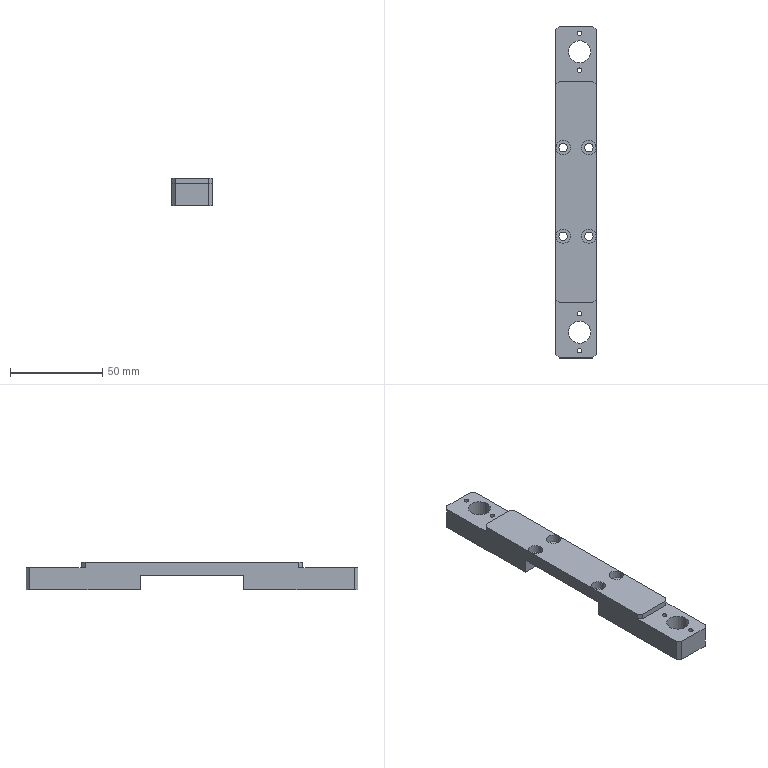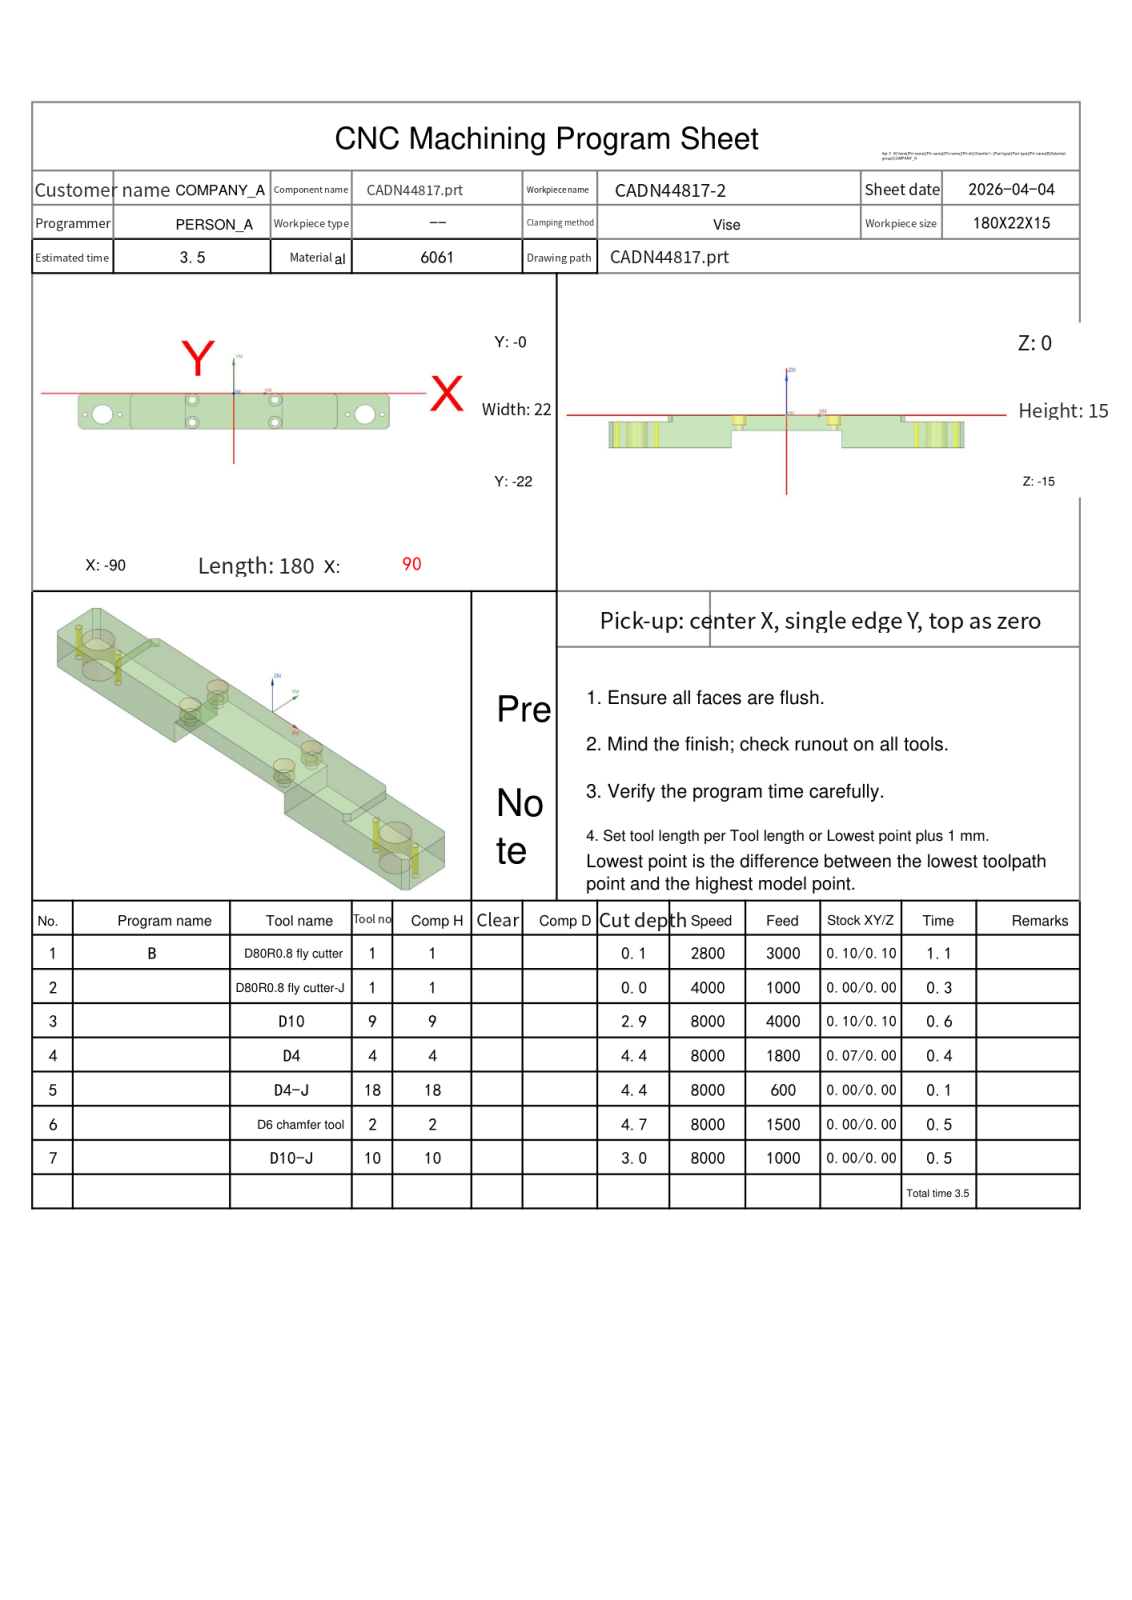NC program | NX | posted by the shop | part box 22 x 180 x 15 mm
Whole program:
%
O0001
(Machine time: 4.85 MIN)
(===Total Tool:6===)
(T1=D80R0.8 fly cutter D=80. R=0.8 D- H01 Z=-0.   )
(T9=D10     D=10.  R=0.   D-  H09 Z=-2.9  )
(T4=D4      D=4.   R=0.   D-  H04 Z=-4.4  )
(T18=D4-J   D=4.   R=0.   D-  H18 Z=-4.4  )
(T2=D6 chamfer tool D=6. R=0. D- H02 Z=-4.75 )
(T10=D10-J  D=10.  R=0.   D10 H10 Z=-3.   )
G80 G90 G17 G49 G40
G91 G28 Z0
M01
N1 T01 M06
(D80R0.8 fly cutter D=80. R=0.8 H=01 ce=0.10 di=0.10)
G00 G90 G54 X-142.097 Y-11. M03 S2800
G43 H01 Z20.
M08
Z6.011
G01 Z4.011 F3000.
X-130.097
X130.097
X142.097
Z6.011
G00 X-142.097
Z5.522
G01 Z3.522
X-130.097
X130.097
X142.097
Z5.522
G00 X-142.097
Z5.033
G01 Z3.033
X-130.097
X130.097
X142.097
Z5.033
G00 X-142.097
Z4.544
G01 Z2.544
X-130.097
X130.097
X142.097
Z4.544
G00 Z20.
X-142.097
Z4.056
G01 Z2.056
X-130.097
X130.097
X142.097
Z4.056
G00 Z20.
X-142.097
Z3.567
G01 Z1.567
X-130.097
X130.097
X142.097
Z3.567
G00 Z20.
X-142.097
Z3.078
G01 Z1.078
X-130.097
X130.097
X142.097
Z3.078
G00 Z20.
X-142.097
Z2.589
G01 Z.589
X-130.097
X130.097
X142.097
Z2.589
G00 Z20.
X-142.097
Z2.1
G01 Z.1
X-130.097
X130.097
X142.097
Z2.1
G00 Z20.
G91 G28 Z0.0
M05
M09
G91 G28 Z0.0
M01
N2 T01 M06
(D80R0.8 fly cutter-J D=80. R=0.8 H=01 ce=0.00 di=0.00)
G00 G90 G54 X-141.999 Y-11. M03 S4000
G43 H01 Z20.
M08
Z2.
G01 Z0.0 F1000.
X-129.999
X129.999
X141.999
Z2.
G00 Z20.
G91 G28 Z0.0
M05
M09
G91 G28 Z0.0
M01
N3 T09 M06
(D10  D=10. R=0. H=09 ce=0.10 di=0.10)
G00 G90 G54 X-92.099 Y-29.209 M03 S8000
G43 H09 Z14.5
M08
Z.92
G01 Z-.58 F4000.
X-92.502 Y-24.427
G02 X-92.6 Y-22.114 I27.402 J2.315
G01 Y.112
G02 X-92.531 Y2.052 I27.5 J0.0
X-92.241 Y2.688 I.997 J-.071
G01 X-90.322 Y4.607
G02 X-89.616 Y4.9 I.707 J-.707
G01 X-88.056
G02 X-87.256 Y4.1 I0.0 J-.8
G01 X-87.268 Y3.963
G03 X-87.6 Y.112 I22.168 J-3.851
G01 Y-22.114
G03 X-87.248 Y-26.076 I22.5 J.002
X-86.264 Y-26.9 I.984 J.176
G01 X-80.258
G03 X-79.559 Y-26.2 I0.0 J.7
G01 X-79.583 Y-26.018
G02 X-80.1 Y-22.114 I14.483 J3.906
G01 Y.112
G02 X-79.541 Y4.171 I15. J0.0
X-78.578 Y4.9 I.963 J-.271
G01 X-71.854
G02 X-71.354 Y4.4 I0.0 J-.5
X-71.432 Y4.132 I-.5 J0.0
G03 X-72.6 Y.112 I6.332 J-4.02
G01 Y-22.112
G03 X-71.127 Y-26.576 I7.5 J0.0
X-70.496 Y-26.966 I.803 J.595
G01 X-61.192 Y-28.592
X-61.02 Y-28.607
G03 X-60.02 Y-27.607 I0.0 J1.
X-60.312 Y-26.9 I-1. J0.0
G01 X-65.1 Y-22.112
Y.112
X-60.312 Y4.9
X-57.112 Y8.1
Z.92
G00 Z14.5
X-92.099 Y-29.209
Z.34
G01 Z-1.16
X-92.502 Y-24.427
G02 X-92.6 Y-22.114 I27.402 J2.315
G01 Y.112
G02 X-92.531 Y2.052 I27.5 J0.0
X-92.241 Y2.688 I.997 J-.071
G01 X-90.322 Y4.607
G02 X-89.616 Y4.9 I.707 J-.707
G01 X-88.056
G02 X-87.256 Y4.1 I0.0 J-.8
G01 X-87.268 Y3.963
G03 X-87.6 Y.112 I22.168 J-3.851
G01 Y-22.114
G03 X-87.248 Y-26.076 I22.5 J.002
X-86.264 Y-26.9 I.984 J.176
G01 X-80.258
G03 X-79.559 Y-26.2 I0.0 J.7
G01 X-79.583 Y-26.018
G02 X-80.1 Y-22.114 I14.483 J3.906
G01 Y.112
G02 X-79.541 Y4.171 I15. J0.0
X-78.578 Y4.9 I.963 J-.271
G01 X-71.854
G02 X-71.354 Y4.4 I0.0 J-.5
X-71.432 Y4.132 I-.5 J0.0
G03 X-72.6 Y.112 I6.332 J-4.02
G01 Y-22.112
G03 X-71.127 Y-26.576 I7.5 J0.0
X-70.496 Y-26.966 I.803 J.595
G01 X-61.192 Y-28.592
X-61.02 Y-28.607
G03 X-60.02 Y-27.607 I0.0 J1.
X-60.312 Y-26.9 I-1. J0.0
G01 X-65.1 Y-22.112
Y.112
X-60.312 Y4.9
X-57.112 Y8.1
Z.34
G00 Z14.5
X-92.099 Y-29.209
Z-.24
G01 Z-1.74
X-92.502 Y-24.427
G02 X-92.6 Y-22.114 I27.402 J2.315
G01 Y.112
G02 X-92.531 Y2.052 I27.5 J0.0
X-92.241 Y2.688 I.997 J-.071
G01 X-90.322 Y4.607
G02 X-89.616 Y4.9 I.707 J-.707
G01 X-88.056
G02 X-87.256 Y4.1 I0.0 J-.8
G01 X-87.268 Y3.963
G03 X-87.6 Y.112 I22.168 J-3.851
G01 Y-22.114
G03 X-87.248 Y-26.076 I22.5 J.002
X-86.264 Y-26.9 I.984 J.176
G01 X-80.258
G03 X-79.559 Y-26.2 I0.0 J.7
G01 X-79.583 Y-26.018
G02 X-80.1 Y-22.114 I14.483 J3.906
G01 Y.112
G02 X-79.541 Y4.171 I15. J0.0
X-78.578 Y4.9 I.963 J-.271
G01 X-71.854
G02 X-71.354 Y4.4 I0.0 J-.5
X-71.432 Y4.132 I-.5 J0.0
G03 X-72.6 Y.112 I6.332 J-4.02
G01 Y-22.112
G03 X-71.127 Y-26.576 I7.5 J0.0
X-70.496 Y-26.966 I.803 J.595
G01 X-61.192 Y-28.592
X-61.02 Y-28.607
G03 X-60.02 Y-27.607 I0.0 J1.
X-60.312 Y-26.9 I-1. J0.0
G01 X-65.1 Y-22.112
Y.112
X-60.312 Y4.9
X-57.112 Y8.1
Z-.24
G00 Z14.5
X-92.099 Y-29.209
Z-.82
G01 Z-2.32
X-92.502 Y-24.427
G02 X-92.6 Y-22.114 I27.402 J2.315
G01 Y.112
G02 X-92.531 Y2.052 I27.5 J0.0
X-92.241 Y2.688 I.997 J-.071
G01 X-90.322 Y4.607
G02 X-89.616 Y4.9 I.707 J-.707
G01 X-88.056
G02 X-87.256 Y4.1 I0.0 J-.8
G01 X-87.268 Y3.963
G03 X-87.6 Y.112 I22.168 J-3.851
G01 Y-22.114
G03 X-87.248 Y-26.076 I22.5 J.002
X-86.264 Y-26.9 I.984 J.176
G01 X-80.258
G03 X-79.559 Y-26.2 I0.0 J.7
G01 X-79.583 Y-26.018
G02 X-80.1 Y-22.114 I14.483 J3.906
G01 Y.112
G02 X-79.541 Y4.171 I15. J0.0
X-78.578 Y4.9 I.963 J-.271
G01 X-71.854
G02 X-71.354 Y4.4 I0.0 J-.5
X-71.432 Y4.132 I-.5 J0.0
G03 X-72.6 Y.112 I6.332 J-4.02
G01 Y-22.112
G03 X-71.127 Y-26.576 I7.5 J0.0
X-70.496 Y-26.966 I.803 J.595
G01 X-61.192 Y-28.592
X-61.02 Y-28.607
G03 X-60.02 Y-27.607 I0.0 J1.
X-60.312 Y-26.9 I-1. J0.0
G01 X-65.1 Y-22.112
Y.112
X-60.312 Y4.9
X-57.112 Y8.1
Z-.82
G00 Z14.5
X-92.099 Y-29.209
Z-1.4
G01 Z-2.9
X-92.502 Y-24.427
G02 X-92.6 Y-22.114 I27.402 J2.315
G01 Y.112
G02 X-92.531 Y2.052 I27.5 J0.0
X-92.241 Y2.688 I.997 J-.071
G01 X-90.322 Y4.607
G02 X-89.616 Y4.9 I.707 J-.707
G01 X-88.056
G02 X-87.256 Y4.1 I0.0 J-.8
G01 X-87.268 Y3.963
G03 X-87.6 Y.112 I22.168 J-3.851
G01 Y-22.114
G03 X-87.248 Y-26.076 I22.5 J.002
X-86.264 Y-26.9 I.984 J.176
G01 X-80.258
G03 X-79.559 Y-26.2 I0.0 J.7
G01 X-79.583 Y-26.018
G02 X-80.1 Y-22.114 I14.483 J3.906
G01 Y.112
G02 X-79.541 Y4.171 I15. J0.0
X-78.578 Y4.9 I.963 J-.271
G01 X-71.854
G02 X-71.354 Y4.4 I0.0 J-.5
X-71.432 Y4.132 I-.5 J0.0
G03 X-72.6 Y.112 I6.332 J-4.02
G01 Y-22.112
G03 X-71.127 Y-26.576 I7.5 J0.0
X-70.496 Y-26.966 I.803 J.595
G01 X-61.192 Y-28.592
X-61.02 Y-28.607
G03 X-60.02 Y-27.607 I0.0 J1.
X-60.312 Y-26.9 I-1. J0.0
G01 X-65.1 Y-22.112
Y.112
X-60.312 Y4.9
X-57.112 Y8.1
Z-1.4
G00 Z3.
X92.099 Y7.209
Z.92
G01 Z-.58
X92.502 Y2.427
G02 X92.6 Y.114 I-27.402 J-2.315
G01 Y-22.112
G02 X92.531 Y-24.052 I-27.5 J0.0
X92.241 Y-24.688 I-.997 J.071
G01 X90.322 Y-26.607
G02 X89.616 Y-26.9 I-.707 J.707
G01 X88.056
G02 X87.256 Y-26.1 I0.0 J.8
G01 X87.268 Y-25.963
G03 X87.6 Y-22.112 I-22.168 J3.851
G01 Y.114
G03 X87.248 Y4.076 I-22.5 J-.002
X86.264 Y4.9 I-.984 J-.176
G01 X80.258
G03 X79.559 Y4.2 I0.0 J-.7
G01 X79.583 Y4.018
G02 X80.1 Y.114 I-14.483 J-3.906
G01 Y-22.112
G02 X79.541 Y-26.171 I-15. J0.0
X78.578 Y-26.9 I-.963 J.271
G01 X71.854
G02 X71.354 Y-26.4 I0.0 J.5
X71.432 Y-26.132 I.5 J0.0
G03 X72.6 Y-22.112 I-6.332 J4.02
G01 Y.112
G03 X71.127 Y4.576 I-7.5 J0.0
X70.496 Y4.966 I-.803 J-.595
G01 X61.192 Y6.592
X61.02 Y6.607
G03 X60.02 Y5.607 I0.0 J-1.
X60.312 Y4.9 I1. J0.0
G01 X65.1 Y.112
Y-22.112
X60.312 Y-26.9
X57.112 Y-30.1
Z.92
G00 Z14.5
X92.099 Y7.209
Z.34
G01 Z-1.16
X92.502 Y2.427
G02 X92.6 Y.114 I-27.402 J-2.315
G01 Y-22.112
G02 X92.531 Y-24.052 I-27.5 J0.0
X92.241 Y-24.688 I-.997 J.071
G01 X90.322 Y-26.607
G02 X89.616 Y-26.9 I-.707 J.707
G01 X88.056
G02 X87.256 Y-26.1 I0.0 J.8
G01 X87.268 Y-25.963
G03 X87.6 Y-22.112 I-22.168 J3.851
G01 Y.114
G03 X87.248 Y4.076 I-22.5 J-.002
X86.264 Y4.9 I-.984 J-.176
G01 X80.258
G03 X79.559 Y4.2 I0.0 J-.7
G01 X79.583 Y4.018
G02 X80.1 Y.114 I-14.483 J-3.906
G01 Y-22.112
G02 X79.541 Y-26.171 I-15. J0.0
X78.578 Y-26.9 I-.963 J.271
G01 X71.854
G02 X71.354 Y-26.4 I0.0 J.5
X71.432 Y-26.132 I.5 J0.0
G03 X72.6 Y-22.112 I-6.332 J4.02
G01 Y.112
G03 X71.127 Y4.576 I-7.5 J0.0
X70.496 Y4.966 I-.803 J-.595
G01 X61.192 Y6.592
X61.02 Y6.607
G03 X60.02 Y5.607 I0.0 J-1.
X60.312 Y4.9 I1. J0.0
G01 X65.1 Y.112
Y-22.112
X60.312 Y-26.9
X57.112 Y-30.1
Z.34
G00 Z14.5
X92.099 Y7.209
Z-.24
G01 Z-1.74
X92.502 Y2.427
G02 X92.6 Y.114 I-27.402 J-2.315
G01 Y-22.112
G02 X92.531 Y-24.052 I-27.5 J0.0
X92.241 Y-24.688 I-.997 J.071
G01 X90.322 Y-26.607
G02 X89.616 Y-26.9 I-.707 J.707
G01 X88.056
G02 X87.256 Y-26.1 I0.0 J.8
G01 X87.268 Y-25.963
G03 X87.6 Y-22.112 I-22.168 J3.851
G01 Y.114
G03 X87.248 Y4.076 I-22.5 J-.002
X86.264 Y4.9 I-.984 J-.176
G01 X80.258
G03 X79.559 Y4.2 I0.0 J-.7
G01 X79.583 Y4.018
G02 X80.1 Y.114 I-14.483 J-3.906
G01 Y-22.112
G02 X79.541 Y-26.171 I-15. J0.0
X78.578 Y-26.9 I-.963 J.271
G01 X71.854
G02 X71.354 Y-26.4 I0.0 J.5
X71.432 Y-26.132 I.5 J0.0
G03 X72.6 Y-22.112 I-6.332 J4.02
G01 Y.112
G03 X71.127 Y4.576 I-7.5 J0.0
X70.496 Y4.966 I-.803 J-.595
G01 X61.192 Y6.592
X61.02 Y6.607
G03 X60.02 Y5.607 I0.0 J-1.
X60.312 Y4.9 I1. J0.0
G01 X65.1 Y.112
Y-22.112
X60.312 Y-26.9
X57.112 Y-30.1
Z-.24
G00 Z14.5
X92.099 Y7.209
Z-.82
G01 Z-2.32
X92.502 Y2.427
G02 X92.6 Y.114 I-27.402 J-2.315
G01 Y-22.112
G02 X92.531 Y-24.052 I-27.5 J0.0
X92.241 Y-24.688 I-.997 J.071
G01 X90.322 Y-26.607
G02 X89.616 Y-26.9 I-.707 J.707
G01 X88.056
G02 X87.256 Y-26.1 I0.0 J.8
G01 X87.268 Y-25.963
G03 X87.6 Y-22.112 I-22.168 J3.851
G01 Y.114
G03 X87.248 Y4.076 I-22.5 J-.002
X86.264 Y4.9 I-.984 J-.176
G01 X80.258
G03 X79.559 Y4.2 I0.0 J-.7
G01 X79.583 Y4.018
G02 X80.1 Y.114 I-14.483 J-3.906
G01 Y-22.112
G02 X79.541 Y-26.171 I-15. J0.0
X78.578 Y-26.9 I-.963 J.271
G01 X71.854
G02 X71.354 Y-26.4 I0.0 J.5
X71.432 Y-26.132 I.5 J0.0
G03 X72.6 Y-22.112 I-6.332 J4.02
G01 Y.112
G03 X71.127 Y4.576 I-7.5 J0.0
X70.496 Y4.966 I-.803 J-.595
G01 X61.192 Y6.592
X61.02 Y6.607
G03 X60.02 Y5.607 I0.0 J-1.
X60.312 Y4.9 I1. J0.0
G01 X65.1 Y.112
Y-22.112
X60.312 Y-26.9
X57.112 Y-30.1
Z-.82
G00 Z14.5
X92.099 Y7.209
Z-1.4
G01 Z-2.9
X92.502 Y2.427
G02 X92.6 Y.114 I-27.402 J-2.315
G01 Y-22.112
G02 X92.531 Y-24.052 I-27.5 J0.0
X92.241 Y-24.688 I-.997 J.071
G01 X90.322 Y-26.607
G02 X89.616 Y-26.9 I-.707 J.707
G01 X88.056
G02 X87.256 Y-26.1 I0.0 J.8
G01 X87.268 Y-25.963
G03 X87.6 Y-22.112 I-22.168 J3.851
G01 Y.114
G03 X87.248 Y4.076 I-22.5 J-.002
X86.264 Y4.9 I-.984 J-.176
G01 X80.258
G03 X79.559 Y4.2 I0.0 J-.7
G01 X79.583 Y4.018
G02 X80.1 Y.114 I-14.483 J-3.906
G01 Y-22.112
G02 X79.541 Y-26.171 I-15. J0.0
X78.578 Y-26.9 I-.963 J.271
G01 X71.854
G02 X71.354 Y-26.4 I0.0 J.5
X71.432 Y-26.132 I.5 J0.0
G03 X72.6 Y-22.112 I-6.332 J4.02
G01 Y.112
G03 X71.127 Y4.576 I-7.5 J0.0
X70.496 Y4.966 I-.803 J-.595
G01 X61.192 Y6.592
X61.02 Y6.607
G03 X60.02 Y5.607 I0.0 J-1.
X60.312 Y4.9 I1. J0.0
G01 X65.1 Y.112
Y-22.112
X60.312 Y-26.9
X57.112 Y-30.1
Z-1.4
G00 Z14.5
G91 G28 Z0.0
M05
M09
G91 G28 Z0.0
M01
N4 T04 M06
(D4  D=4. R=0. H=04 ce=0.07 di=0.00)
G00 G90 G54 X-24. Y-4. M03 S8000
G43 H04 Z20.
M08
Z.3
G03 X-24.915 Y-4.915 I0.0 J-.915 F1800.
X-24. Y-5.83 I.915 J0.0
X-24. Y-5.83 Z-.05 I0.0 J1.83
X-24. Y-5.83 Z-.4 I0.0 J1.83
X-24. Y-5.83 Z-.75 I0.0 J1.83
X-24. Y-5.83 Z-1.1 I0.0 J1.83
X-24. Y-5.83 Z-1.45 I0.0 J1.83
X-24. Y-5.83 Z-1.8 I0.0 J1.83
X-24. Y-5.83 Z-2.15 I0.0 J1.83
X-24. Y-5.83 Z-2.5 I0.0 J1.83
X-24. Y-5.83 Z-2.85 I0.0 J1.83
X-24. Y-5.83 Z-3.2 I0.0 J1.83
X-24. Y-5.83 Z-3.55 I0.0 J1.83
X-24. Y-5.83 Z-3.9 I0.0 J1.83
X-24. Y-5.83 Z-4.25 I0.0 J1.83
X-23.206 Y-2.351 Z-4.4 I0.0 J1.83
X-24. Y-2.17 I-.794 J-1.649
X-25.83 Y-4. I0.0 J-1.83
X-24. Y-5.83 I1.83 J0.0
X-22.17 Y-4. I0.0 J1.83
X-23.206 Y-2.351 I-1.83 J0.0
X-23.603 Y-2.261 I-.397 J-.824
X-24.518 Y-3.176 I0.0 J-.915
X-24. Y-4. I.915 J0.0
G00 Z20.
Y-18.
Z.3
G03 X-24.915 Y-18.915 I0.0 J-.915
X-24. Y-19.83 I.915 J0.0
X-24. Y-19.83 Z-.05 I0.0 J1.83
X-24. Y-19.83 Z-.4 I0.0 J1.83
X-24. Y-19.83 Z-.75 I0.0 J1.83
X-24. Y-19.83 Z-1.1 I0.0 J1.83
X-24. Y-19.83 Z-1.45 I0.0 J1.83
X-24. Y-19.83 Z-1.8 I0.0 J1.83
X-24. Y-19.83 Z-2.15 I0.0 J1.83
X-24. Y-19.83 Z-2.5 I0.0 J1.83
X-24. Y-19.83 Z-2.85 I0.0 J1.83
X-24. Y-19.83 Z-3.2 I0.0 J1.83
X-24. Y-19.83 Z-3.55 I0.0 J1.83
X-24. Y-19.83 Z-3.9 I0.0 J1.83
X-24. Y-19.83 Z-4.25 I0.0 J1.83
X-23.206 Y-16.351 Z-4.4 I0.0 J1.83
X-24. Y-16.17 I-.794 J-1.649
X-25.83 Y-18. I0.0 J-1.83
X-24. Y-19.83 I1.83 J0.0
X-22.17 Y-18. I0.0 J1.83
X-23.206 Y-16.351 I-1.83 J0.0
X-23.603 Y-16.261 I-.397 J-.824
X-24.518 Y-17.176 I0.0 J-.915
X-24. Y-18. I.915 J0.0
G00 Z20.
X24.
Z.3
G03 X23.085 Y-18.915 I0.0 J-.915
X24. Y-19.83 I.915 J0.0
X24. Y-19.83 Z-.05 I0.0 J1.83
X24. Y-19.83 Z-.4 I0.0 J1.83
X24. Y-19.83 Z-.75 I0.0 J1.83
X24. Y-19.83 Z-1.1 I0.0 J1.83
X24. Y-19.83 Z-1.45 I0.0 J1.83
X24. Y-19.83 Z-1.8 I0.0 J1.83
X24. Y-19.83 Z-2.15 I0.0 J1.83
X24. Y-19.83 Z-2.5 I0.0 J1.83
X24. Y-19.83 Z-2.85 I0.0 J1.83
X24. Y-19.83 Z-3.2 I0.0 J1.83
X24. Y-19.83 Z-3.55 I0.0 J1.83
X24. Y-19.83 Z-3.9 I0.0 J1.83
X24. Y-19.83 Z-4.25 I0.0 J1.83
X24.794 Y-16.351 Z-4.4 I0.0 J1.83
X24. Y-16.17 I-.794 J-1.649
X22.17 Y-18. I0.0 J-1.83
X24. Y-19.83 I1.83 J0.0
X25.83 Y-18. I0.0 J1.83
X24.794 Y-16.351 I-1.83 J0.0
X24.397 Y-16.261 I-.397 J-.824
X23.482 Y-17.176 I0.0 J-.915
X24. Y-18. I.915 J0.0
G00 Z20.
Y-4.
Z.3
G03 X23.085 Y-4.915 I0.0 J-.915
X24. Y-5.83 I.915 J0.0
X24. Y-5.83 Z-.05 I0.0 J1.83
X24. Y-5.83 Z-.4 I0.0 J1.83
X24. Y-5.83 Z-.75 I0.0 J1.83
X24. Y-5.83 Z-1.1 I0.0 J1.83
X24. Y-5.83 Z-1.45 I0.0 J1.83
X24. Y-5.83 Z-1.8 I0.0 J1.83
X24. Y-5.83 Z-2.15 I0.0 J1.83
X24. Y-5.83 Z-2.5 I0.0 J1.83
X24. Y-5.83 Z-2.85 I0.0 J1.83
X24. Y-5.83 Z-3.2 I0.0 J1.83
X24. Y-5.83 Z-3.55 I0.0 J1.83
X24. Y-5.83 Z-3.9 I0.0 J1.83
X24. Y-5.83 Z-4.25 I0.0 J1.83
X24.794 Y-2.351 Z-4.4 I0.0 J1.83
X24. Y-2.17 I-.794 J-1.649
X22.17 Y-4. I0.0 J-1.83
X24. Y-5.83 I1.83 J0.0
X25.83 Y-4. I0.0 J1.83
X24.794 Y-2.351 I-1.83 J0.0
X24.397 Y-2.261 I-.397 J-.824
X23.482 Y-3.176 I0.0 J-.915
X24. Y-4. I.915 J0.0
G00 Z20.
G91 G28 Z0.0
M05
M09
G91 G28 Z0.0
M01
N5 T18 M06
(D4-J  D=4. R=0. H=18 ce=0.00 di=0.00)
G00 G90 G54 X-24. Y-4. M03 S8000
G43 H18 Z20.
M08
Z-4.4
G01 X-24.326 Y-5.495 F600.
X-24.334 Y-5.566
G03 X-24. Y-5.9 I.334 J0.0
X-22.1 Y-4. I0.0 J1.9
X-24. Y-2.1 I-1.9 J0.0
X-25.9 Y-4. I0.0 J-1.9
X-24. Y-5.9 I1.9 J0.0
X-23.506 Y-5.835 I0.0 J1.9
X-23.259 Y-5.512 I-.087 J.322
G01 X-23.296 Y-5.358
X-24. Y-4.
G00 Z20.
Y-18.
Z-4.4
G01 X-24.326 Y-19.495
X-24.334 Y-19.566
G03 X-24. Y-19.9 I.334 J0.0
X-22.1 Y-18. I0.0 J1.9
X-24. Y-16.1 I-1.9 J0.0
X-25.9 Y-18. I0.0 J-1.9
X-24. Y-19.9 I1.9 J0.0
X-23.506 Y-19.835 I0.0 J1.9
X-23.259 Y-19.512 I-.087 J.322
G01 X-23.296 Y-19.358
X-24. Y-18.
G00 Z20.
X24.
Z-4.4
G01 X23.674 Y-19.495
X23.666 Y-19.566
G03 X24. Y-19.9 I.334 J0.0
X25.9 Y-18. I0.0 J1.9
X24. Y-16.1 I-1.9 J0.0
X22.1 Y-18. I0.0 J-1.9
X24. Y-19.9 I1.9 J0.0
X24.494 Y-19.835 I0.0 J1.9
X24.741 Y-19.512 I-.087 J.322
G01 X24.704 Y-19.358
X24. Y-18.
G00 Z20.
Y-4.
Z-4.4
G01 X23.674 Y-5.495
X23.666 Y-5.566
G03 X24. Y-5.9 I.334 J0.0
X25.9 Y-4. I0.0 J1.9
X24. Y-2.1 I-1.9 J0.0
X22.1 Y-4. I0.0 J-1.9
X24. Y-5.9 I1.9 J0.0
X24.494 Y-5.835 I0.0 J1.9
X24.741 Y-5.512 I-.087 J.322
G01 X24.704 Y-5.358
X24. Y-4.
G00 Z20.
G91 G28 Z0.0
M05
M09
G91 G28 Z0.0
M01
N6 T02 M06
(D6 chamfer tool D=6. R=0. H=02 ce=0.00 di=0.00)
G00 G90 G54 X-86. Y-13. M03 S8000
G43 H02 Z20.
M08
G98 G81 X-86. Y-13. Z-4.75 R0.0 F1000.
X-66.
X66.
X86.
G80
G00 Z20.
G00 G90 X.386 Y-23.127 M03 S8000
Z20.
Z.272
G01 Z-1.2 F1350.
G03 X.1 Y-22.927 I-1.286 J-1.532
G01 X.054 Y-22.897
X0.0 Y-22.9
X-58. F1500.
X-58.233 Y-22.869
X-58.45 Y-22.779
X-58.636 Y-22.636
X-60.636 Y-20.636
X-60.779 Y-20.45
X-60.869 Y-20.233
X-60.9 Y-20.
Y-2.
X-60.869 Y-1.767
X-60.779 Y-1.55
X-60.636 Y-1.364
X-58.636 Y.636
X-58.45 Y.779
X-58.233 Y.869
X-58. Y.9
X58.
X58.233 Y.869
X58.45 Y.779
X58.636 Y.636
X60.636 Y-1.364
X60.779 Y-1.55
X60.869 Y-1.767
X60.9 Y-2.
Y-20.
X60.869 Y-20.233
X60.779 Y-20.45
X60.636 Y-20.636
X58.636 Y-22.636
X58.45 Y-22.779
X58.233 Y-22.869
X58. Y-22.9
X0.0
X-.054 Y-22.897
X-.1 Y-22.927
G03 X-.386 Y-23.127 I1. J-1.732
G01 Z.272
G00 Z10.
X-23.599 Y-15.197
Z.333
G01 Z-1.2 F1350.
G03 X-23.898 Y-15.019 I-1.167 J-1.624
G01 X-23.946 Y-14.993
X-24. Y-15.
G03 X-27. Y-18. I0.0 J-3. F1500.
X-24. Y-21. I3. J0.0
X-21. Y-18. I0.0 J3.
X-24. Y-15. I-3. J0.0
G01 X-24.054 Y-14.993
X-24.102 Y-15.019
G03 X-24.401 Y-15.197 I.868 J-1.802
G01 Z.333
G00 Z10.
X-23.599 Y-1.197
Z.333
G01 Z-1.2 F1350.
G03 X-23.898 Y-1.019 I-1.167 J-1.624
G01 X-23.946 Y-.993
X-24. Y-1.
G03 X-27. Y-4. I0.0 J-3. F1500.
X-24. Y-7. I3. J0.0
X-21. Y-4. I0.0 J3.
X-24. Y-1. I-3. J0.0
G01 X-24.054 Y-.993
X-24.102 Y-1.019
G03 X-24.401 Y-1.197 I.868 J-1.802
G01 Z.333
G00 Z10.
X24.401
Z.333
G01 Z-1.2 F1350.
G03 X24.102 Y-1.019 I-1.167 J-1.624
G01 X24.054 Y-.993
X24. Y-1.
G03 X21. Y-4. I0.0 J-3. F1500.
X24. Y-7. I3. J0.0
X27. Y-4. I0.0 J3.
X24. Y-1. I-3. J0.0
G01 X23.946 Y-.993
X23.898 Y-1.019
G03 X23.599 Y-1.197 I.868 J-1.802
G01 Z.333
G00 Z10.
X24.401 Y-15.197
Z.333
G01 Z-1.2 F1350.
G03 X24.102 Y-15.019 I-1.167 J-1.624
G01 X24.054 Y-14.993
X24. Y-15.
G03 X21. Y-18. I0.0 J-3. F1500.
X24. Y-21. I3. J0.0
X27. Y-18. I0.0 J3.
X24. Y-15. I-3. J0.0
G01 X23.946 Y-14.993
X23.898 Y-15.019
G03 X23.599 Y-15.197 I.868 J-1.802
G01 Z.333
G00 Z10.
X61.442 Y1.081
Z-1.8
G01 Z-4.2 F1350.
G03 X61.67 Y.921 I1.028 J1.226
G01 X61.706 Y.896
X61.75 Y.9
X88. F1500.
X88.233 Y.869
X88.45 Y.779
X88.636 Y.636
X90.636 Y-1.364
X90.779 Y-1.55
X90.869 Y-1.767
X90.9 Y-2.
Y-20.
X90.869 Y-20.233
X90.779 Y-20.45
X90.636 Y-20.636
X88.636 Y-22.636
X88.45 Y-22.779
X88.233 Y-22.869
X88. Y-22.9
X61.75
X61.706 Y-22.896
X61.67 Y-22.921
G03 X61.442 Y-23.081 I.8 J-1.386
G01 Z-1.8
G00 Z10.
X76.398 Y-8.104
Z-2.682
G01 Z-4.2 F1350.
G03 X76.101 Y-7.921 I-1.194 J-1.604
G01 X76.054 Y-7.894
X76. Y-7.9
G03 X70.9 Y-13. I0.0 J-5.1 F1500.
X76. Y-18.1 I5.1 J0.0
X81.1 Y-13. I0.0 J5.1
X76. Y-7.9 I-5.1 J0.0
G01 X75.946 Y-7.894
X75.899 Y-7.921
G03 X75.602 Y-8.104 I.898 J-1.787
G01 Z-2.682
G00 Z10.
X-61.442 Y-23.081
Z-1.8
G01 Z-4.2 F1350.
G03 X-61.67 Y-22.921 I-1.028 J-1.226
G01 X-61.706 Y-22.896
X-61.75 Y-22.9
X-88. F1500.
X-88.233 Y-22.869
X-88.45 Y-22.779
X-88.636 Y-22.636
X-90.636 Y-20.636
X-90.779 Y-20.45
X-90.869 Y-20.233
X-90.9 Y-20.
Y-2.
X-90.869 Y-1.767
X-90.779 Y-1.55
X-90.636 Y-1.364
X-88.636 Y.636
X-88.45 Y.779
X-88.233 Y.869
X-88. Y.9
X-61.75
X-61.706 Y.896
X-61.67 Y.921
G03 X-61.442 Y1.081 I-.8 J1.386
G01 Z-1.8
G00 Z10.
X-75.602 Y-8.104
Z-2.682
G01 Z-4.2 F1350.
G03 X-75.899 Y-7.921 I-1.194 J-1.604
G01 X-75.946 Y-7.894
X-76. Y-7.9
G03 X-81.1 Y-13. I0.0 J-5.1 F1500.
X-76. Y-18.1 I5.1 J0.0
X-70.9 Y-13. I0.0 J5.1
X-76. Y-7.9 I-5.1 J0.0
G01 X-76.054 Y-7.894
X-76.101 Y-7.921
G03 X-76.398 Y-8.104 I.898 J-1.787
G01 Z-2.682
G00 Z20.
G91 G28 Z0.0
M05
M09
G91 G28 Z0.0
M01
N7 T10 M06
(D10-J  D=10. R=0. H=10 ce=0.40 di=0.00)
G00 G90 G54 X-96.407 Y1.014 M03 S8000
G43 H10 Z14.5
M08
Z-1.5
G01 Z-3. F1000.
X-92.4
G02 X-90.4 Y-.986 I0.0 J-2.
G01 Y-20.6
G03 X-90.107 Y-21.307 I1. J0.0
G01 X-88.707 Y-22.707
G03 X-88. Y-23. I.707 J.707
G01 X-86.3
G03 X-85.4 Y-22.1 I0.0 J.9
G01 Y0.0
G02 X-84.4 Y1. I1. J0.0
G01 X-81.3
G02 X-80.4 Y.1 I0.0 J-.9
G01 Y-22.
G03 X-79.4 Y-23. I1. J0.0
G01 X-76.3
G03 X-75.4 Y-22.1 I0.0 J.9
G01 Y.1
G02 X-74.5 Y1. I.9 J0.0
G01 X-71.3
G02 X-70.4 Y.1 I0.0 J-.9
G01 Y-22.237
Y-22.282
G03 X-69.734 Y-23.215 I1. J.009
G01 X-65.677 Y-24.65
G03 X-65.344 Y-24.707 I.333 J.943
X-64.344 Y-23.707 I0.0 J1.
X-64.637 Y-23. I-1. J0.0
G01 X-65.4 Y-22.237
Y.237
X-64.637 Y1.
G03 X-64.051 Y2.414 I-1.414 J1.414
X-64.637 Y3.828 I-2. J0.0
G01 X-67.808 Y7.
Z-1.5
G00 Z14.5
X96.407 Y-23.014
Z-1.5
G01 Z-3.
X92.4
G02 X90.4 Y-21.014 I0.0 J2.
G01 Y-1.4
G03 X90.107 Y-.693 I-1. J0.0
G01 X88.707 Y.707
G03 X88. Y1. I-.707 J-.707
G01 X86.3
G03 X85.4 Y.1 I0.0 J-.9
G01 Y-22.
G02 X84.4 Y-23. I-1. J0.0
G01 X81.3
G02 X80.4 Y-22.1 I0.0 J.9
G01 Y0.0
G03 X79.4 Y1. I-1. J0.0
G01 X76.3
G03 X75.4 Y.1 I0.0 J-.9
G01 Y-22.1
G02 X74.5 Y-23. I-.9 J0.0
G01 X71.3
G02 X70.4 Y-22.1 I0.0 J.9
G01 Y.237
Y.282
G03 X69.734 Y1.215 I-1. J-.009
G01 X65.677 Y2.65
G03 X65.344 Y2.707 I-.333 J-.943
X64.344 Y1.707 I0.0 J-1.
X64.637 Y1. I1. J0.0
G01 X65.4 Y.237
Y-22.237
X64.637 Y-23.
G03 X64.051 Y-24.414 I1.414 J-1.414
X64.637 Y-25.828 I2. J0.0
G01 X67.808 Y-29.
Z-1.5
G00 Z14.5
G00 G90 X-59.632 Y-29.191 M03 S8000
Z14.5
Z-2.
G01 Z-3. F1000.
G41 D10
X-59.573 Y-29.
G03 X-59.485 Y-28.414 I-1.912 J.586
X-60.071 Y-27. I-2. J0.0
G01 X-65. Y-22.071
Y.071
X-60.071 Y5.
G03 X-59.485 Y6.414 I-1.414 J1.414
X-59.573 Y7. I-2. J0.0
G01 G40 X-59.632 Y7.191
Z-2.
G00 Z2.
X59.632
Z-2.
G01 Z-3.
G41 D10
X59.573 Y7.
G03 X59.485 Y6.414 I1.912 J-.586
X60.071 Y5. I2. J0.0
G01 X65. Y.071
Y-22.071
X60.071 Y-27.
G03 X59.485 Y-28.414 I1.414 J-1.414
X59.573 Y-29. I2. J0.0
G01 G40 X59.632 Y-29.191
Z-2.
G00 Z14.5
M05
M09
G91 G28 Z0.0
G91 G28 Y0.0
M30
%